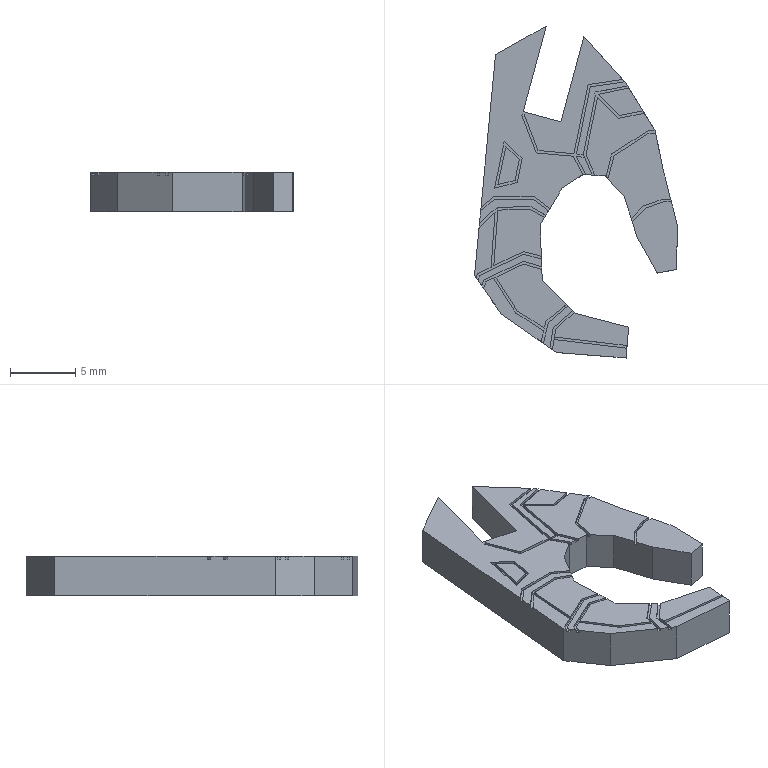Part | SolidWorks | features BaseBody 1 | 1 solid | 148 faces | box 15.584 x 25.481 x 3 mm | volume 593.723 mm3 | plane 128 | spline 20